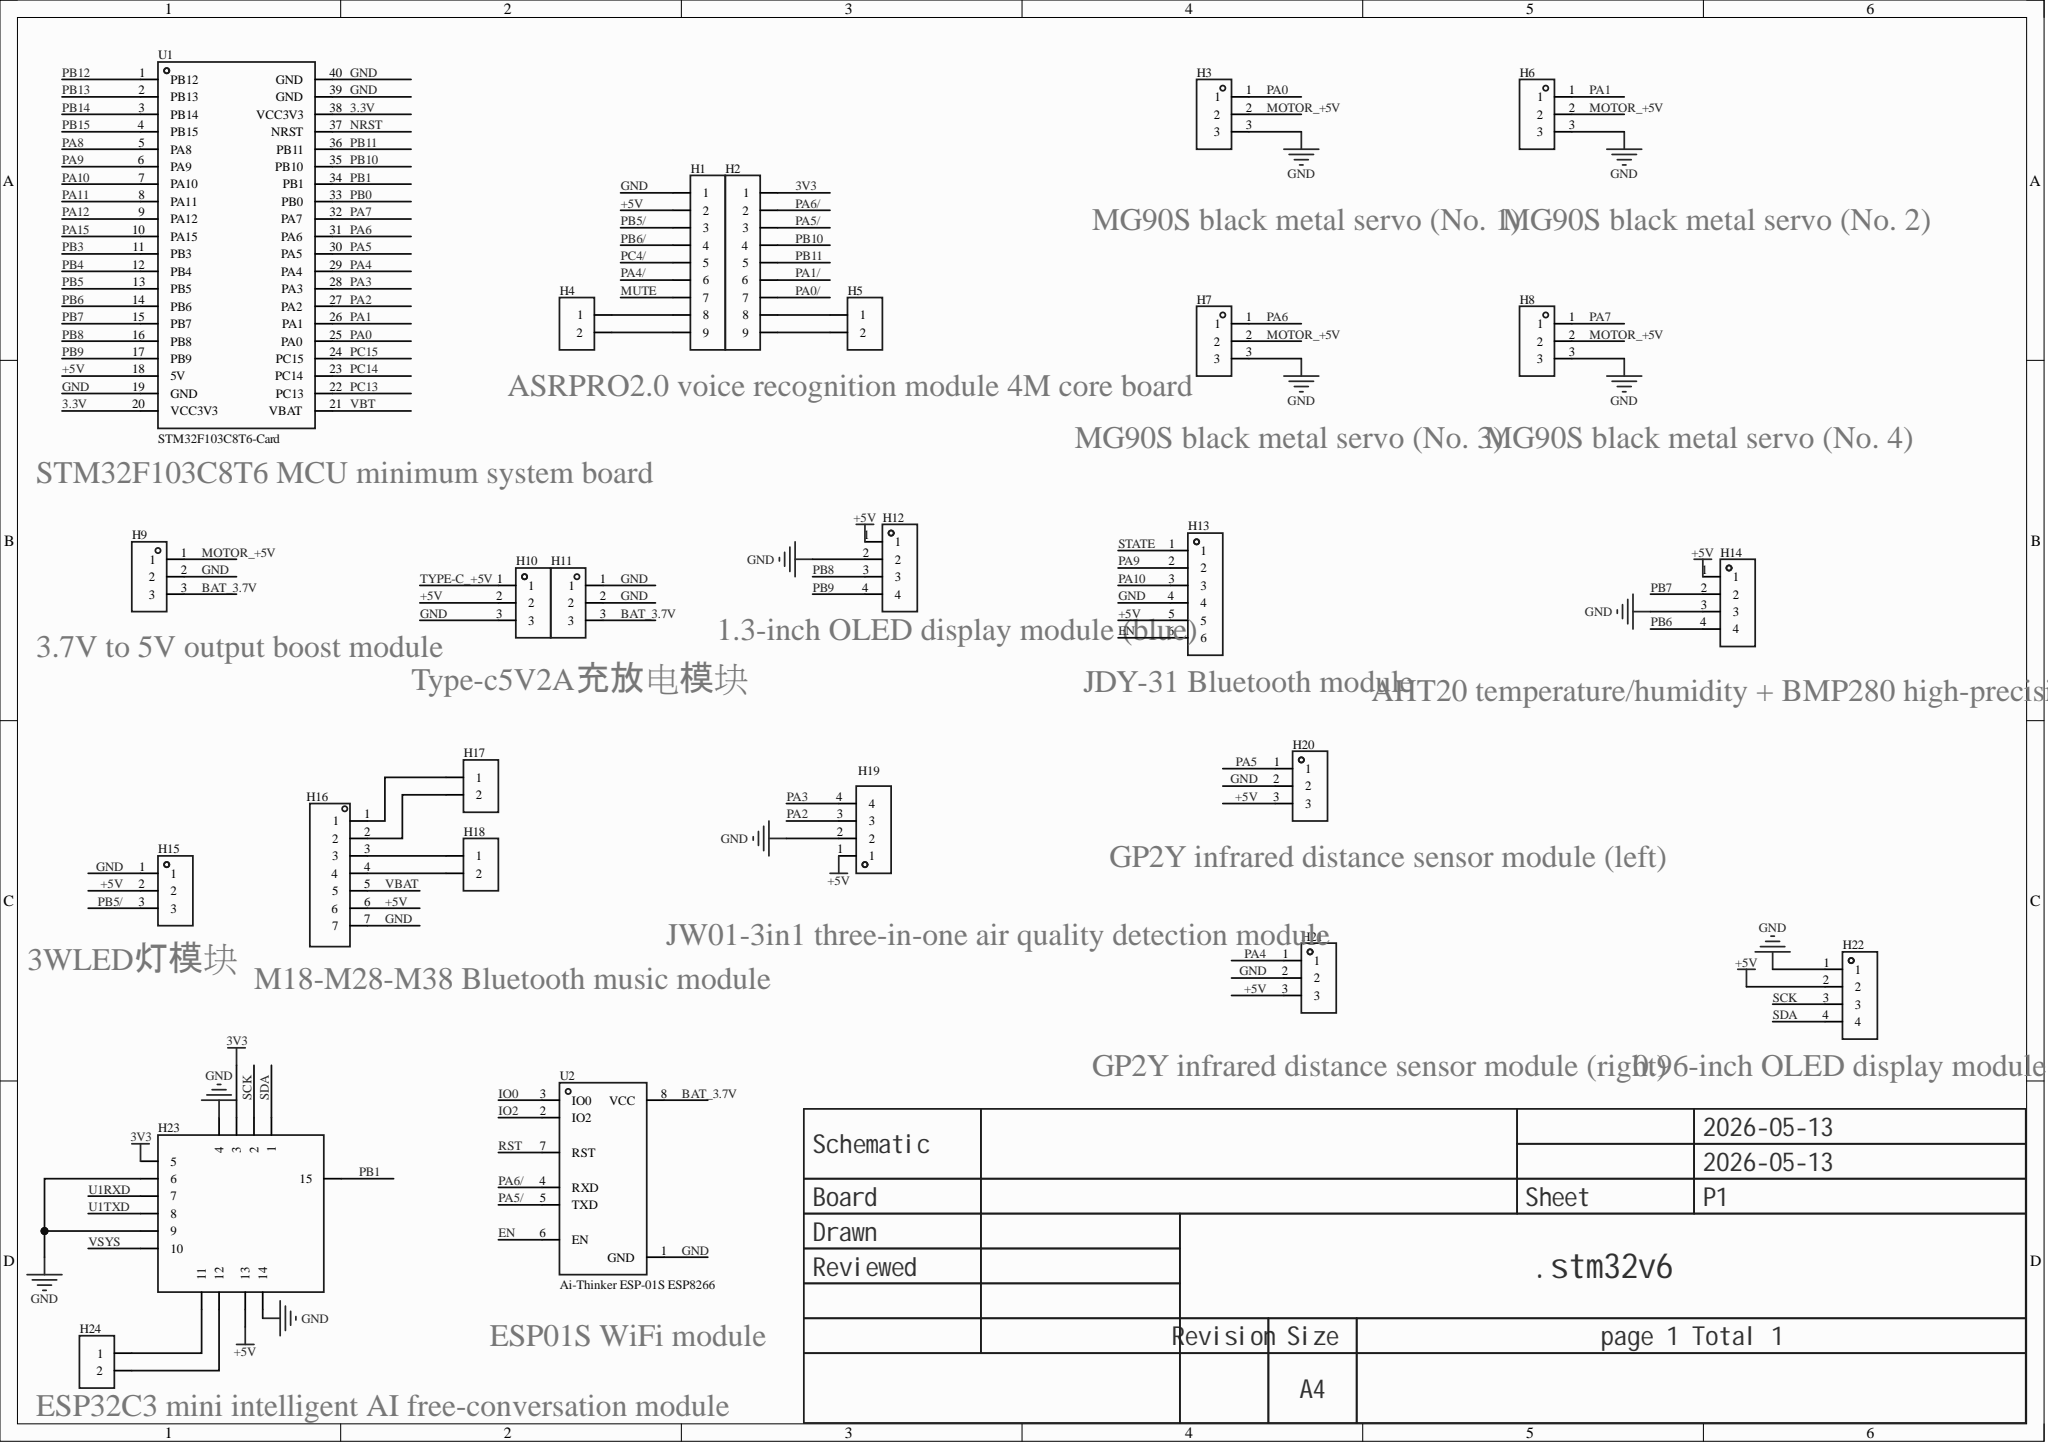Circuit board | Altium Designer | 26 parts | 39 nets
Bill of materials:
Comment,Description,Designator,Footprint,LibRef,Quantity
"","","H1, H2","HDR-TH_9P-P2.54-V-F-1","HDR-F_2.54_1x9P","2"
"","","H3, H6, H7, H8, H9, H10, H11, H15, H20, H21","HDR-TH_3P-P2.54-V-F","HDR-F_2.54_1x3P","10"
"","","H4, H5, H17, H18, H24","HDR-TH_2P-P2.54-V-F","HDR-F_2.54_1x2P","5"
"","","H12, H14, H19, H22","HDR-TH_4P-P2.54-V-F","HDR-F_2.54_1x4P","4"
"","","H13","HDR-TH_6P-P2.54-V-F","HDR-F_2.54_1x6P","1"
"","","H16","HDR-TH_7P-P2.54-V-F","HDR-F_2.54_1x7P","1"
"","","H23","ESP32C3MINI","HDR-F_2.54_2x8","1"
"STM32F103C8T6-Card","","U1","CONN-TH_L53.3-W22.9_STM32F103C8T6-CARD","STM32F103C8T6-Card","1"
"Ai-Thinker ESP-01S ESP8266","","U2","WIFIM-TH_8P-L24.7-W14.4-P2.54","Ai-Thinker ESP-01S ESP8266","1"
Netlist (Protel format):
[
H1
HDR-TH_9P-P2.54-V-F-1




]
[
H2
HDR-TH_9P-P2.54-V-F-1




]
[
H3
HDR-TH_3P-P2.54-V-F




]
[
H4
HDR-TH_2P-P2.54-V-F




]
[
H5
HDR-TH_2P-P2.54-V-F




]
[
H6
HDR-TH_3P-P2.54-V-F




]
[
H7
HDR-TH_3P-P2.54-V-F




]
[
H8
HDR-TH_3P-P2.54-V-F




]
[
H9
HDR-TH_3P-P2.54-V-F




]
[
H10
HDR-TH_3P-P2.54-V-F




]
[
H11
HDR-TH_3P-P2.54-V-F




]
[
H12
HDR-TH_4P-P2.54-V-F




]
[
H13
HDR-TH_6P-P2.54-V-F




]
[
H14
HDR-TH_4P-P2.54-V-F




]
[
H15
HDR-TH_3P-P2.54-V-F




]
[
H16
HDR-TH_7P-P2.54-V-F




]
[
H17
HDR-TH_2P-P2.54-V-F




]
[
H18
HDR-TH_2P-P2.54-V-F




]
[
H19
HDR-TH_4P-P2.54-V-F




]
[
H20
HDR-TH_3P-P2.54-V-F




]
[
H21
HDR-TH_3P-P2.54-V-F




]
[
H22
HDR-TH_4P-P2.54-V-F




]
[
H23
ESP32C3MINI




]
[
H24
HDR-TH_2P-P2.54-V-F




]
[
U1
CONN-TH_L53.3-W22.9_STM32F103C8T6-CARD
STM32F103C8T6-Card



]
[
U2
WIFIM-TH_8P-L24.7-W14.4-P2.54
Ai-Thinker ESP-01S ESP8266



]
(
SDA
H22-4
H23-1
)
(
SCK
H22-3
H23-2
)
(
PB11
H2-5
U1-36
)
(
PB10
H2-4
U1-35
)
(
PB9
H12-4
U1-17
)
(
PB8
H12-3
U1-16
)
(
PB7
H14-2
U1-15
)
(
PB6
H14-4
U1-14
)
(
PB5/
H1-3
H15-3
)
(
PB1
H23-15
U1-34
)
(
PA10
H13-3
U1-7
)
(
PA9
H13-2
U1-6
)
(
PA7
H8-1
U1-32
)
(
PA6/
H2-2
U2-4
)
(
PA6
H7-1
U1-31
)
(
PA5/
H2-3
U2-5
)
(
PA5
H20-1
U1-30
)
(
PA4
H21-1
U1-29
)
(
PA3
H19-4
U1-28
)
(
PA2
H19-3
U1-27
)
(
PA1
H6-1
U1-26
)
(
PA0
H3-1
U1-25
)
(
NetH23_12
H23-12
H24-2
)
(
NetH23_11
H23-11
H24-1
)
(
NetH16_4
H16-4
H18-2
)
(
NetH16_3
H16-3
H18-1
)
(
NetH16_2
H16-2
H17-2
)
(
NetH16_1
H16-1
H17-1
)
(
NetH2_9
H2-9
H5-2
)
(
NetH2_8
H2-8
H5-1
)
(
NetH1_9
H1-9
H4-2
)
(
NetH1_8
H1-8
H4-1
)
(
MOTOR_+5V
H3-2
H6-2
H7-2
H8-2
H9-1
)
(
GND
H1-1
H3-3
H6-3
H7-3
H8-3
H9-2
H10-3
H11-1
H11-2
H12-2
H13-4
H14-3
H15-1
H16-7
H19-2
H20-2
H21-2
H22-1
H23-4
H23-6
H23-9
H23-14
U1-19
U1-39
U1-40
U2-1
)
(
EN
H13-6
U2-6
)
(
BAT_3.7V
H9-3
H11-3
U2-8
)
(
+5V
H1-2
H10-2
H12-1
H13-5
H14-1
H15-2
H16-6
H19-1
H20-3
H21-3
H22-2
H23-13
U1-18
)
(
3V3
H2-1
H23-3
H23-5
)
(
3.3V
U1-20
U1-38
)